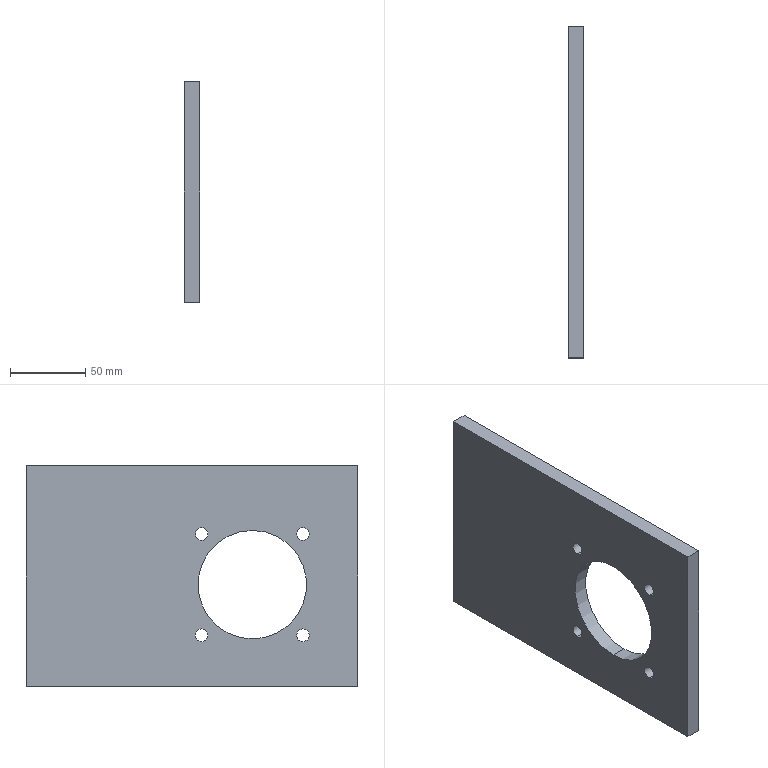Part | SolidWorks | features BaseBody 1 | 1 solid | 16 faces | box 10 x 220 x 146 mm | volume 278281 mm3 | cylinder 10 | plane 6 | commonest cylinder face diameters 8.376 x8 72 x2
STEP:
#1=CARTESIAN_POINT('',(-136.129,135.83,5.011));
#2=VERTEX_POINT('',#1);
#3=CARTESIAN_POINT('',(-136.129,135.83,77.011));
#4=VERTEX_POINT('',#3);
#5=CARTESIAN_POINT('',(-136.129,135.83,41.011));
#6=DIRECTION('',(-1.,0.,0.));
#7=DIRECTION('',(0.,0.,1.));
#8=AXIS2_PLACEMENT_3D('',#5,#6,#7);
#9=CIRCLE('',#8,36.);
#10=EDGE_CURVE('',#2,#4,#9,.T.);
#11=ORIENTED_EDGE('',*,*,#10,.F.);
#12=CARTESIAN_POINT('',(-146.129,135.83,5.011));
#13=VERTEX_POINT('',#12);
#14=CARTESIAN_POINT('',(-136.129,135.83,5.011));
#15=DIRECTION('',(-1.,0.,0.));
#16=VECTOR('',#15,1000.);
#17=LINE('',#14,#16);
#18=EDGE_CURVE('',#2,#13,#17,.T.);
#19=ORIENTED_EDGE('',*,*,#18,.T.);
#20=CARTESIAN_POINT('',(-146.129,135.83,77.011));
#21=VERTEX_POINT('',#20);
#22=CARTESIAN_POINT('',(-146.129,135.83,41.011));
#23=DIRECTION('',(-1.,0.,0.));
#24=DIRECTION('',(0.,0.,1.));
#25=AXIS2_PLACEMENT_3D('',#22,#23,#24);
#26=CIRCLE('',#25,36.);
#27=EDGE_CURVE('',#13,#21,#26,.T.);
#28=ORIENTED_EDGE('',*,*,#27,.T.);
#29=CARTESIAN_POINT('',(-136.129,135.83,77.011));
#30=DIRECTION('',(-1.,0.,0.));
#31=VECTOR('',#30,1000.);
#32=LINE('',#29,#31);
#33=EDGE_CURVE('',#4,#21,#32,.T.);
#34=ORIENTED_EDGE('',*,*,#33,.F.);
#35=EDGE_LOOP('',(#11,#19,#28,#34));
#36=FACE_OUTER_BOUND('',#35,.T.);
#37=CARTESIAN_POINT('',(-136.129,135.83,41.011));
#38=DIRECTION('',(-1.,0.,0.));
#39=DIRECTION('',(0.,0.,1.));
#40=AXIS2_PLACEMENT_3D('',#37,#38,#39);
#41=CYLINDRICAL_SURFACE('',#40,36.);
#42=ADVANCED_FACE('',(#36),#41,.F.);
#43=CARTESIAN_POINT('',(-146.129,169.417,3.235));
#44=VERTEX_POINT('',#43);
#45=CARTESIAN_POINT('',(-146.129,169.417,11.611));
#46=VERTEX_POINT('',#45);
#47=CARTESIAN_POINT('',(-146.129,169.417,7.423));
#48=DIRECTION('',(-1.,0.,0.));
#49=DIRECTION('',(0.,0.,-1.));
#50=AXIS2_PLACEMENT_3D('',#47,#48,#49);
#51=CIRCLE('',#50,4.188);
#52=EDGE_CURVE('',#44,#46,#51,.T.);
#53=ORIENTED_EDGE('',*,*,#52,.T.);
#54=CARTESIAN_POINT('',(-136.129,169.417,11.611));
#55=VERTEX_POINT('',#54);
#56=CARTESIAN_POINT('',(-400.356,169.417,11.611));
#57=DIRECTION('',(1.,0.,0.));
#58=VECTOR('',#57,1000.);
#59=LINE('',#56,#58);
#60=EDGE_CURVE('',#46,#55,#59,.T.);
#61=ORIENTED_EDGE('',*,*,#60,.T.);
#62=CARTESIAN_POINT('',(-136.129,169.417,3.235));
#63=VERTEX_POINT('',#62);
#64=CARTESIAN_POINT('',(-136.129,169.417,7.423));
#65=DIRECTION('',(-1.,0.,0.));
#66=DIRECTION('',(0.,0.,-1.));
#67=AXIS2_PLACEMENT_3D('',#64,#65,#66);
#68=CIRCLE('',#67,4.188);
#69=EDGE_CURVE('',#63,#55,#68,.T.);
#70=ORIENTED_EDGE('',*,*,#69,.F.);
#71=CARTESIAN_POINT('',(-400.356,169.417,3.235));
#72=DIRECTION('',(1.,0.,0.));
#73=VECTOR('',#72,1000.);
#74=LINE('',#71,#73);
#75=EDGE_CURVE('',#44,#63,#74,.T.);
#76=ORIENTED_EDGE('',*,*,#75,.F.);
#77=EDGE_LOOP('',(#53,#61,#70,#76));
#78=FACE_OUTER_BOUND('',#77,.T.);
#79=CARTESIAN_POINT('',(-400.356,169.417,7.423));
#80=DIRECTION('',(1.,0.,0.));
#81=DIRECTION('',(0.,0.,-1.));
#82=AXIS2_PLACEMENT_3D('',#79,#80,#81);
#83=CYLINDRICAL_SURFACE('',#82,4.188);
#84=ADVANCED_FACE('',(#78),#83,.F.);
#85=CARTESIAN_POINT('',(-146.129,102.242,3.235));
#86=VERTEX_POINT('',#85);
#87=CARTESIAN_POINT('',(-146.129,102.242,11.611));
#88=VERTEX_POINT('',#87);
#89=CARTESIAN_POINT('',(-146.129,102.242,7.423));
#90=DIRECTION('',(-1.,0.,0.));
#91=DIRECTION('',(0.,0.,-1.));
#92=AXIS2_PLACEMENT_3D('',#89,#90,#91);
#93=CIRCLE('',#92,4.188);
#94=EDGE_CURVE('',#86,#88,#93,.T.);
#95=ORIENTED_EDGE('',*,*,#94,.T.);
#96=CARTESIAN_POINT('',(-136.129,102.242,11.611));
#97=VERTEX_POINT('',#96);
#98=CARTESIAN_POINT('',(-400.356,102.242,11.611));
#99=DIRECTION('',(1.,0.,0.));
#100=VECTOR('',#99,1000.);
#101=LINE('',#98,#100);
#102=EDGE_CURVE('',#88,#97,#101,.T.);
#103=ORIENTED_EDGE('',*,*,#102,.T.);
#104=CARTESIAN_POINT('',(-136.129,102.242,3.235));
#105=VERTEX_POINT('',#104);
#106=CARTESIAN_POINT('',(-136.129,102.242,7.423));
#107=DIRECTION('',(-1.,0.,0.));
#108=DIRECTION('',(0.,0.,-1.));
#109=AXIS2_PLACEMENT_3D('',#106,#107,#108);
#110=CIRCLE('',#109,4.188);
#111=EDGE_CURVE('',#105,#97,#110,.T.);
#112=ORIENTED_EDGE('',*,*,#111,.F.);
#113=CARTESIAN_POINT('',(-400.356,102.242,3.235));
#114=DIRECTION('',(1.,0.,0.));
#115=VECTOR('',#114,1000.);
#116=LINE('',#113,#115);
#117=EDGE_CURVE('',#86,#105,#116,.T.);
#118=ORIENTED_EDGE('',*,*,#117,.F.);
#119=EDGE_LOOP('',(#95,#103,#112,#118));
#120=FACE_OUTER_BOUND('',#119,.T.);
#121=CARTESIAN_POINT('',(-400.356,102.242,7.423));
#122=DIRECTION('',(1.,0.,0.));
#123=DIRECTION('',(0.,0.,-1.));
#124=AXIS2_PLACEMENT_3D('',#121,#122,#123);
#125=CYLINDRICAL_SURFACE('',#124,4.188);
#126=ADVANCED_FACE('',(#120),#125,.F.);
#127=CARTESIAN_POINT('',(-146.129,102.242,70.41));
#128=VERTEX_POINT('',#127);
#129=CARTESIAN_POINT('',(-146.129,102.242,78.786));
#130=VERTEX_POINT('',#129);
#131=CARTESIAN_POINT('',(-146.129,102.242,74.598));
#132=DIRECTION('',(-1.,0.,0.));
#133=DIRECTION('',(0.,0.,-1.));
#134=AXIS2_PLACEMENT_3D('',#131,#132,#133);
#135=CIRCLE('',#134,4.188);
#136=EDGE_CURVE('',#128,#130,#135,.T.);
#137=ORIENTED_EDGE('',*,*,#136,.T.);
#138=CARTESIAN_POINT('',(-136.129,102.242,78.786));
#139=VERTEX_POINT('',#138);
#140=CARTESIAN_POINT('',(-400.356,102.242,78.786));
#141=DIRECTION('',(1.,0.,0.));
#142=VECTOR('',#141,1000.);
#143=LINE('',#140,#142);
#144=EDGE_CURVE('',#130,#139,#143,.T.);
#145=ORIENTED_EDGE('',*,*,#144,.T.);
#146=CARTESIAN_POINT('',(-136.129,102.242,70.41));
#147=VERTEX_POINT('',#146);
#148=CARTESIAN_POINT('',(-136.129,102.242,74.598));
#149=DIRECTION('',(-1.,0.,0.));
#150=DIRECTION('',(0.,0.,-1.));
#151=AXIS2_PLACEMENT_3D('',#148,#149,#150);
#152=CIRCLE('',#151,4.188);
#153=EDGE_CURVE('',#147,#139,#152,.T.);
#154=ORIENTED_EDGE('',*,*,#153,.F.);
#155=CARTESIAN_POINT('',(-400.356,102.242,70.41));
#156=DIRECTION('',(1.,0.,0.));
#157=VECTOR('',#156,1000.);
#158=LINE('',#155,#157);
#159=EDGE_CURVE('',#128,#147,#158,.T.);
#160=ORIENTED_EDGE('',*,*,#159,.F.);
#161=EDGE_LOOP('',(#137,#145,#154,#160));
#162=FACE_OUTER_BOUND('',#161,.T.);
#163=CARTESIAN_POINT('',(-400.356,102.242,74.598));
#164=DIRECTION('',(1.,0.,0.));
#165=DIRECTION('',(0.,0.,-1.));
#166=AXIS2_PLACEMENT_3D('',#163,#164,#165);
#167=CYLINDRICAL_SURFACE('',#166,4.188);
#168=ADVANCED_FACE('',(#162),#167,.F.);
#169=CARTESIAN_POINT('',(-146.129,169.417,70.41));
#170=VERTEX_POINT('',#169);
#171=CARTESIAN_POINT('',(-146.129,169.417,78.786));
#172=VERTEX_POINT('',#171);
#173=CARTESIAN_POINT('',(-146.129,169.417,74.598));
#174=DIRECTION('',(-1.,0.,0.));
#175=DIRECTION('',(0.,0.,-1.));
#176=AXIS2_PLACEMENT_3D('',#173,#174,#175);
#177=CIRCLE('',#176,4.188);
#178=EDGE_CURVE('',#170,#172,#177,.T.);
#179=ORIENTED_EDGE('',*,*,#178,.T.);
#180=CARTESIAN_POINT('',(-136.129,169.417,78.786));
#181=VERTEX_POINT('',#180);
#182=CARTESIAN_POINT('',(-400.356,169.417,78.786));
#183=DIRECTION('',(1.,0.,0.));
#184=VECTOR('',#183,1000.);
#185=LINE('',#182,#184);
#186=EDGE_CURVE('',#172,#181,#185,.T.);
#187=ORIENTED_EDGE('',*,*,#186,.T.);
#188=CARTESIAN_POINT('',(-136.129,169.417,70.41));
#189=VERTEX_POINT('',#188);
#190=CARTESIAN_POINT('',(-136.129,169.417,74.598));
#191=DIRECTION('',(-1.,0.,0.));
#192=DIRECTION('',(0.,0.,-1.));
#193=AXIS2_PLACEMENT_3D('',#190,#191,#192);
#194=CIRCLE('',#193,4.188);
#195=EDGE_CURVE('',#189,#181,#194,.T.);
#196=ORIENTED_EDGE('',*,*,#195,.F.);
#197=CARTESIAN_POINT('',(-400.356,169.417,70.41));
#198=DIRECTION('',(1.,0.,0.));
#199=VECTOR('',#198,1000.);
#200=LINE('',#197,#199);
#201=EDGE_CURVE('',#170,#189,#200,.T.);
#202=ORIENTED_EDGE('',*,*,#201,.F.);
#203=EDGE_LOOP('',(#179,#187,#196,#202));
#204=FACE_OUTER_BOUND('',#203,.T.);
#205=CARTESIAN_POINT('',(-400.356,169.417,74.598));
#206=DIRECTION('',(1.,0.,0.));
#207=DIRECTION('',(0.,0.,-1.));
#208=AXIS2_PLACEMENT_3D('',#205,#206,#207);
#209=CYLINDRICAL_SURFACE('',#208,4.188);
#210=ADVANCED_FACE('',(#204),#209,.F.);
#211=CARTESIAN_POINT('',(-146.129,135.83,41.011));
#212=DIRECTION('',(-1.,0.,0.));
#213=DIRECTION('',(0.,0.,1.));
#214=AXIS2_PLACEMENT_3D('',#211,#212,#213);
#215=CIRCLE('',#214,36.);
#216=EDGE_CURVE('',#21,#13,#215,.T.);
#217=ORIENTED_EDGE('',*,*,#216,.F.);
#218=ORIENTED_EDGE('',*,*,#27,.F.);
#219=EDGE_LOOP('',(#217,#218));
#220=FACE_BOUND('',#219,.T.);
#221=ORIENTED_EDGE('',*,*,#52,.F.);
#222=CARTESIAN_POINT('',(-146.129,169.417,7.423));
#223=DIRECTION('',(-1.,0.,0.));
#224=DIRECTION('',(0.,0.,-1.));
#225=AXIS2_PLACEMENT_3D('',#222,#223,#224);
#226=CIRCLE('',#225,4.188);
#227=EDGE_CURVE('',#46,#44,#226,.T.);
#228=ORIENTED_EDGE('',*,*,#227,.F.);
#229=EDGE_LOOP('',(#221,#228));
#230=FACE_BOUND('',#229,.T.);
#231=ORIENTED_EDGE('',*,*,#94,.F.);
#232=CARTESIAN_POINT('',(-146.129,102.242,7.423));
#233=DIRECTION('',(-1.,0.,0.));
#234=DIRECTION('',(0.,0.,-1.));
#235=AXIS2_PLACEMENT_3D('',#232,#233,#234);
#236=CIRCLE('',#235,4.188);
#237=EDGE_CURVE('',#88,#86,#236,.T.);
#238=ORIENTED_EDGE('',*,*,#237,.F.);
#239=EDGE_LOOP('',(#231,#238));
#240=FACE_BOUND('',#239,.T.);
#241=ORIENTED_EDGE('',*,*,#136,.F.);
#242=CARTESIAN_POINT('',(-146.129,102.242,74.598));
#243=DIRECTION('',(-1.,0.,0.));
#244=DIRECTION('',(0.,0.,-1.));
#245=AXIS2_PLACEMENT_3D('',#242,#243,#244);
#246=CIRCLE('',#245,4.188);
#247=EDGE_CURVE('',#130,#128,#246,.T.);
#248=ORIENTED_EDGE('',*,*,#247,.F.);
#249=EDGE_LOOP('',(#241,#248));
#250=FACE_BOUND('',#249,.T.);
#251=ORIENTED_EDGE('',*,*,#178,.F.);
#252=CARTESIAN_POINT('',(-146.129,169.417,74.598));
#253=DIRECTION('',(-1.,0.,0.));
#254=DIRECTION('',(0.,0.,-1.));
#255=AXIS2_PLACEMENT_3D('',#252,#253,#254);
#256=CIRCLE('',#255,4.188);
#257=EDGE_CURVE('',#172,#170,#256,.T.);
#258=ORIENTED_EDGE('',*,*,#257,.F.);
#259=EDGE_LOOP('',(#251,#258));
#260=FACE_BOUND('',#259,.T.);
#261=CARTESIAN_POINT('',(-146.129,285.83,-26.239));
#262=VERTEX_POINT('',#261);
#263=CARTESIAN_POINT('',(-146.129,285.83,119.761));
#264=VERTEX_POINT('',#263);
#265=CARTESIAN_POINT('',(-146.129,285.83,46.761));
#266=DIRECTION('',(0.,0.,1.));
#267=VECTOR('',#266,1000.);
#268=LINE('',#265,#267);
#269=EDGE_CURVE('',#262,#264,#268,.T.);
#270=ORIENTED_EDGE('',*,*,#269,.F.);
#271=CARTESIAN_POINT('',(-146.129,65.83,-26.239));
#272=VERTEX_POINT('',#271);
#273=CARTESIAN_POINT('',(-146.129,175.83,-26.239));
#274=DIRECTION('',(0.,1.,0.));
#275=VECTOR('',#274,1000.);
#276=LINE('',#273,#275);
#277=EDGE_CURVE('',#272,#262,#276,.T.);
#278=ORIENTED_EDGE('',*,*,#277,.F.);
#279=CARTESIAN_POINT('',(-146.129,65.83,119.761));
#280=VERTEX_POINT('',#279);
#281=CARTESIAN_POINT('',(-146.129,65.83,46.761));
#282=DIRECTION('',(0.,0.,-1.));
#283=VECTOR('',#282,1000.);
#284=LINE('',#281,#283);
#285=EDGE_CURVE('',#280,#272,#284,.T.);
#286=ORIENTED_EDGE('',*,*,#285,.F.);
#287=CARTESIAN_POINT('',(-146.129,175.83,119.761));
#288=DIRECTION('',(0.,-1.,0.));
#289=VECTOR('',#288,1000.);
#290=LINE('',#287,#289);
#291=EDGE_CURVE('',#264,#280,#290,.T.);
#292=ORIENTED_EDGE('',*,*,#291,.F.);
#293=EDGE_LOOP('',(#270,#278,#286,#292));
#294=FACE_OUTER_BOUND('',#293,.T.);
#295=CARTESIAN_POINT('',(-146.129,175.83,46.761));
#296=DIRECTION('',(1.,0.,0.));
#297=DIRECTION('',(0.,0.,-1.));
#298=AXIS2_PLACEMENT_3D('',#295,#296,#297);
#299=PLANE('',#298);
#300=ADVANCED_FACE('',(#220,#230,#240,#250,#260,#294),#299,.F.);
#301=ORIENTED_EDGE('',*,*,#18,.F.);
#302=CARTESIAN_POINT('',(-136.129,135.83,41.011));
#303=DIRECTION('',(-1.,0.,0.));
#304=DIRECTION('',(0.,0.,1.));
#305=AXIS2_PLACEMENT_3D('',#302,#303,#304);
#306=CIRCLE('',#305,36.);
#307=EDGE_CURVE('',#4,#2,#306,.T.);
#308=ORIENTED_EDGE('',*,*,#307,.F.);
#309=ORIENTED_EDGE('',*,*,#33,.T.);
#310=ORIENTED_EDGE('',*,*,#216,.T.);
#311=EDGE_LOOP('',(#301,#308,#309,#310));
#312=FACE_OUTER_BOUND('',#311,.T.);
#313=CARTESIAN_POINT('',(-136.129,135.83,41.011));
#314=DIRECTION('',(-1.,0.,0.));
#315=DIRECTION('',(0.,0.,1.));
#316=AXIS2_PLACEMENT_3D('',#313,#314,#315);
#317=CYLINDRICAL_SURFACE('',#316,36.);
#318=ADVANCED_FACE('',(#312),#317,.F.);
#319=ORIENTED_EDGE('',*,*,#60,.F.);
#320=ORIENTED_EDGE('',*,*,#227,.T.);
#321=ORIENTED_EDGE('',*,*,#75,.T.);
#322=CARTESIAN_POINT('',(-136.129,169.417,7.423));
#323=DIRECTION('',(-1.,0.,0.));
#324=DIRECTION('',(0.,0.,-1.));
#325=AXIS2_PLACEMENT_3D('',#322,#323,#324);
#326=CIRCLE('',#325,4.188);
#327=EDGE_CURVE('',#55,#63,#326,.T.);
#328=ORIENTED_EDGE('',*,*,#327,.F.);
#329=EDGE_LOOP('',(#319,#320,#321,#328));
#330=FACE_OUTER_BOUND('',#329,.T.);
#331=CARTESIAN_POINT('',(-400.356,169.417,7.423));
#332=DIRECTION('',(1.,0.,0.));
#333=DIRECTION('',(0.,0.,-1.));
#334=AXIS2_PLACEMENT_3D('',#331,#332,#333);
#335=CYLINDRICAL_SURFACE('',#334,4.188);
#336=ADVANCED_FACE('',(#330),#335,.F.);
#337=ORIENTED_EDGE('',*,*,#102,.F.);
#338=ORIENTED_EDGE('',*,*,#237,.T.);
#339=ORIENTED_EDGE('',*,*,#117,.T.);
#340=CARTESIAN_POINT('',(-136.129,102.242,7.423));
#341=DIRECTION('',(-1.,0.,0.));
#342=DIRECTION('',(0.,0.,-1.));
#343=AXIS2_PLACEMENT_3D('',#340,#341,#342);
#344=CIRCLE('',#343,4.188);
#345=EDGE_CURVE('',#97,#105,#344,.T.);
#346=ORIENTED_EDGE('',*,*,#345,.F.);
#347=EDGE_LOOP('',(#337,#338,#339,#346));
#348=FACE_OUTER_BOUND('',#347,.T.);
#349=CARTESIAN_POINT('',(-400.356,102.242,7.423));
#350=DIRECTION('',(1.,0.,0.));
#351=DIRECTION('',(0.,0.,-1.));
#352=AXIS2_PLACEMENT_3D('',#349,#350,#351);
#353=CYLINDRICAL_SURFACE('',#352,4.188);
#354=ADVANCED_FACE('',(#348),#353,.F.);
#355=ORIENTED_EDGE('',*,*,#144,.F.);
#356=ORIENTED_EDGE('',*,*,#247,.T.);
#357=ORIENTED_EDGE('',*,*,#159,.T.);
#358=CARTESIAN_POINT('',(-136.129,102.242,74.598));
#359=DIRECTION('',(-1.,0.,0.));
#360=DIRECTION('',(0.,0.,-1.));
#361=AXIS2_PLACEMENT_3D('',#358,#359,#360);
#362=CIRCLE('',#361,4.188);
#363=EDGE_CURVE('',#139,#147,#362,.T.);
#364=ORIENTED_EDGE('',*,*,#363,.F.);
#365=EDGE_LOOP('',(#355,#356,#357,#364));
#366=FACE_OUTER_BOUND('',#365,.T.);
#367=CARTESIAN_POINT('',(-400.356,102.242,74.598));
#368=DIRECTION('',(1.,0.,0.));
#369=DIRECTION('',(0.,0.,-1.));
#370=AXIS2_PLACEMENT_3D('',#367,#368,#369);
#371=CYLINDRICAL_SURFACE('',#370,4.188);
#372=ADVANCED_FACE('',(#366),#371,.F.);
#373=ORIENTED_EDGE('',*,*,#186,.F.);
#374=ORIENTED_EDGE('',*,*,#257,.T.);
#375=ORIENTED_EDGE('',*,*,#201,.T.);
#376=CARTESIAN_POINT('',(-136.129,169.417,74.598));
#377=DIRECTION('',(-1.,0.,0.));
#378=DIRECTION('',(0.,0.,-1.));
#379=AXIS2_PLACEMENT_3D('',#376,#377,#378);
#380=CIRCLE('',#379,4.188);
#381=EDGE_CURVE('',#181,#189,#380,.T.);
#382=ORIENTED_EDGE('',*,*,#381,.F.);
#383=EDGE_LOOP('',(#373,#374,#375,#382));
#384=FACE_OUTER_BOUND('',#383,.T.);
#385=CARTESIAN_POINT('',(-400.356,169.417,74.598));
#386=DIRECTION('',(1.,0.,0.));
#387=DIRECTION('',(0.,0.,-1.));
#388=AXIS2_PLACEMENT_3D('',#385,#386,#387);
#389=CYLINDRICAL_SURFACE('',#388,4.188);
#390=ADVANCED_FACE('',(#384),#389,.F.);
#391=ORIENTED_EDGE('',*,*,#291,.T.);
#392=CARTESIAN_POINT('',(-136.129,65.83,119.761));
#393=VERTEX_POINT('',#392);
#394=CARTESIAN_POINT('',(-146.129,65.83,119.761));
#395=DIRECTION('',(1.,0.,0.));
#396=VECTOR('',#395,1000.);
#397=LINE('',#394,#396);
#398=EDGE_CURVE('',#280,#393,#397,.T.);
#399=ORIENTED_EDGE('',*,*,#398,.T.);
#400=CARTESIAN_POINT('',(-136.129,285.83,119.761));
#401=VERTEX_POINT('',#400);
#402=CARTESIAN_POINT('',(-136.129,65.83,119.761));
#403=DIRECTION('',(0.,1.,0.));
#404=VECTOR('',#403,1000.);
#405=LINE('',#402,#404);
#406=EDGE_CURVE('',#393,#401,#405,.T.);
#407=ORIENTED_EDGE('',*,*,#406,.T.);
#408=CARTESIAN_POINT('',(-146.129,285.83,119.761));
#409=DIRECTION('',(-1.,0.,0.));
#410=VECTOR('',#409,1000.);
#411=LINE('',#408,#410);
#412=EDGE_CURVE('',#401,#264,#411,.T.);
#413=ORIENTED_EDGE('',*,*,#412,.T.);
#414=EDGE_LOOP('',(#391,#399,#407,#413));
#415=FACE_OUTER_BOUND('',#414,.T.);
#416=CARTESIAN_POINT('',(-146.129,65.83,119.761));
#417=DIRECTION('',(0.,0.,1.));
#418=DIRECTION('',(1.,0.,0.));
#419=AXIS2_PLACEMENT_3D('',#416,#417,#418);
#420=PLANE('',#419);
#421=ADVANCED_FACE('',(#415),#420,.T.);
#422=ORIENTED_EDGE('',*,*,#269,.T.);
#423=ORIENTED_EDGE('',*,*,#412,.F.);
#424=CARTESIAN_POINT('',(-136.129,285.83,-26.239));
#425=VERTEX_POINT('',#424);
#426=CARTESIAN_POINT('',(-136.129,285.83,119.761));
#427=DIRECTION('',(0.,0.,-1.));
#428=VECTOR('',#427,1000.);
#429=LINE('',#426,#428);
#430=EDGE_CURVE('',#401,#425,#429,.T.);
#431=ORIENTED_EDGE('',*,*,#430,.T.);
#432=CARTESIAN_POINT('',(-146.129,285.83,-26.239));
#433=DIRECTION('',(-1.,0.,0.));
#434=VECTOR('',#433,1000.);
#435=LINE('',#432,#434);
#436=EDGE_CURVE('',#425,#262,#435,.T.);
#437=ORIENTED_EDGE('',*,*,#436,.T.);
#438=EDGE_LOOP('',(#422,#423,#431,#437));
#439=FACE_OUTER_BOUND('',#438,.T.);
#440=CARTESIAN_POINT('',(-146.129,285.83,119.761));
#441=DIRECTION('',(0.,1.,0.));
#442=DIRECTION('',(0.,0.,1.));
#443=AXIS2_PLACEMENT_3D('',#440,#441,#442);
#444=PLANE('',#443);
#445=ADVANCED_FACE('',(#439),#444,.T.);
#446=ORIENTED_EDGE('',*,*,#277,.T.);
#447=ORIENTED_EDGE('',*,*,#436,.F.);
#448=CARTESIAN_POINT('',(-136.129,65.83,-26.239));
#449=VERTEX_POINT('',#448);
#450=CARTESIAN_POINT('',(-136.129,285.83,-26.239));
#451=DIRECTION('',(0.,-1.,0.));
#452=VECTOR('',#451,1000.);
#453=LINE('',#450,#452);
#454=EDGE_CURVE('',#425,#449,#453,.T.);
#455=ORIENTED_EDGE('',*,*,#454,.T.);
#456=CARTESIAN_POINT('',(-146.129,65.83,-26.239));
#457=DIRECTION('',(-1.,0.,0.));
#458=VECTOR('',#457,1000.);
#459=LINE('',#456,#458);
#460=EDGE_CURVE('',#449,#272,#459,.T.);
#461=ORIENTED_EDGE('',*,*,#460,.T.);
#462=EDGE_LOOP('',(#446,#447,#455,#461));
#463=FACE_OUTER_BOUND('',#462,.T.);
#464=CARTESIAN_POINT('',(-146.129,285.83,-26.239));
#465=DIRECTION('',(0.,0.,-1.));
#466=DIRECTION('',(-1.,0.,0.));
#467=AXIS2_PLACEMENT_3D('',#464,#465,#466);
#468=PLANE('',#467);
#469=ADVANCED_FACE('',(#463),#468,.T.);
#470=ORIENTED_EDGE('',*,*,#285,.T.);
#471=ORIENTED_EDGE('',*,*,#460,.F.);
#472=CARTESIAN_POINT('',(-136.129,65.83,-26.239));
#473=DIRECTION('',(0.,0.,1.));
#474=VECTOR('',#473,1000.);
#475=LINE('',#472,#474);
#476=EDGE_CURVE('',#449,#393,#475,.T.);
#477=ORIENTED_EDGE('',*,*,#476,.T.);
#478=ORIENTED_EDGE('',*,*,#398,.F.);
#479=EDGE_LOOP('',(#470,#471,#477,#478));
#480=FACE_OUTER_BOUND('',#479,.T.);
#481=CARTESIAN_POINT('',(-146.129,65.83,-26.239));
#482=DIRECTION('',(0.,-1.,0.));
#483=DIRECTION('',(0.,0.,-1.));
#484=AXIS2_PLACEMENT_3D('',#481,#482,#483);
#485=PLANE('',#484);
#486=ADVANCED_FACE('',(#480),#485,.T.);
#487=ORIENTED_EDGE('',*,*,#307,.T.);
#488=ORIENTED_EDGE('',*,*,#10,.T.);
#489=EDGE_LOOP('',(#487,#488));
#490=FACE_BOUND('',#489,.T.);
#491=ORIENTED_EDGE('',*,*,#69,.T.);
#492=ORIENTED_EDGE('',*,*,#327,.T.);
#493=EDGE_LOOP('',(#491,#492));
#494=FACE_BOUND('',#493,.T.);
#495=ORIENTED_EDGE('',*,*,#111,.T.);
#496=ORIENTED_EDGE('',*,*,#345,.T.);
#497=EDGE_LOOP('',(#495,#496));
#498=FACE_BOUND('',#497,.T.);
#499=ORIENTED_EDGE('',*,*,#153,.T.);
#500=ORIENTED_EDGE('',*,*,#363,.T.);
#501=EDGE_LOOP('',(#499,#500));
#502=FACE_BOUND('',#501,.T.);
#503=ORIENTED_EDGE('',*,*,#195,.T.);
#504=ORIENTED_EDGE('',*,*,#381,.T.);
#505=EDGE_LOOP('',(#503,#504));
#506=FACE_BOUND('',#505,.T.);
#507=ORIENTED_EDGE('',*,*,#476,.F.);
#508=ORIENTED_EDGE('',*,*,#454,.F.);
#509=ORIENTED_EDGE('',*,*,#430,.F.);
#510=ORIENTED_EDGE('',*,*,#406,.F.);
#511=EDGE_LOOP('',(#507,#508,#509,#510));
#512=FACE_OUTER_BOUND('',#511,.T.);
#513=CARTESIAN_POINT('',(-136.129,175.83,46.761));
#514=DIRECTION('',(1.,0.,0.));
#515=DIRECTION('',(0.,0.,-1.));
#516=AXIS2_PLACEMENT_3D('',#513,#514,#515);
#517=PLANE('',#516);
#518=ADVANCED_FACE('',(#490,#494,#498,#502,#506,#512),#517,.T.);
#519=CLOSED_SHELL('',(#42,#84,#126,#168,#210,#300,#318,#336,#354,#372,#390,#421,#445,#469,#486,#518));
#520=MANIFOLD_SOLID_BREP('',#519);
#521=CARTESIAN_POINT('',(0.,0.,0.));
#522=DIRECTION('',(0.,0.,1.));
#523=DIRECTION('',(1.,0.,0.));
#524=AXIS2_PLACEMENT_3D('',#521,#522,#523);
#525=(LENGTH_UNIT()NAMED_UNIT(*)SI_UNIT(.MILLI.,.METRE.));
#526=UNCERTAINTY_MEASURE_WITH_UNIT(LENGTH_MEASURE(0.00001),#525,'','');
#527=(NAMED_UNIT(*)PLANE_ANGLE_UNIT()SI_UNIT($,.RADIAN.));
#528=(NAMED_UNIT(*)SI_UNIT($,.STERADIAN.)SOLID_ANGLE_UNIT());
#529=(GEOMETRIC_REPRESENTATION_CONTEXT(3)GLOBAL_UNCERTAINTY_ASSIGNED_CONTEXT((#526))GLOBAL_UNIT_ASSIGNED_CONTEXT((#525,#527,#528))REPRESENTATION_CONTEXT('',''));
#530=ADVANCED_BREP_SHAPE_REPRESENTATION('',(#520,#524),#529);